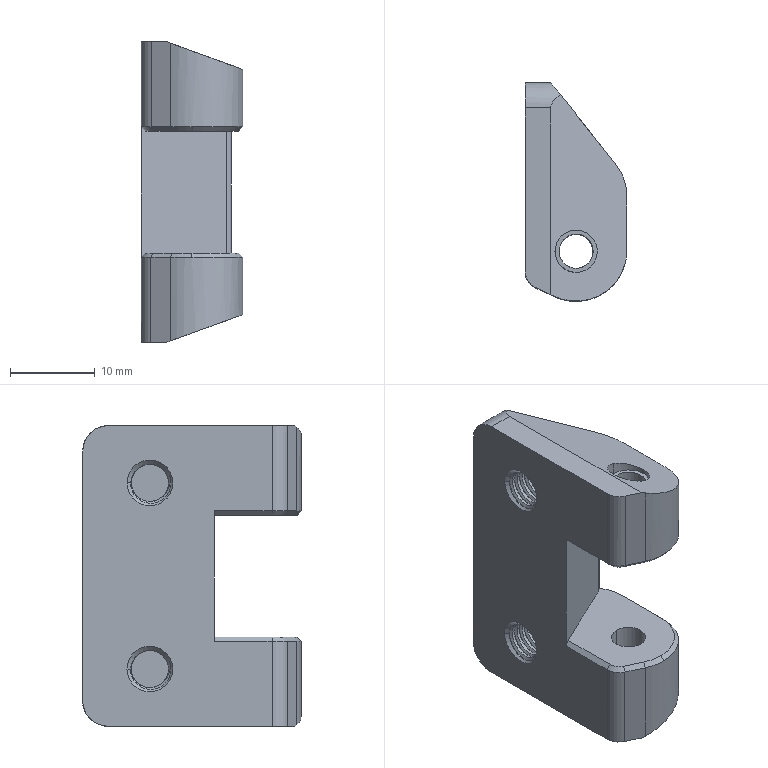Part | SolidWorks | features BaseBody 1 | 1 solid | 142 faces | box 12.027 x 25.816 x 35.476 mm | volume 5447 mm3 | cylinder 90 | plane 30 | cone 18 | spline 4 | commonest cylinder face diameters 5 x44 4.4 x31 4.03 x6 12 x4 4 x2 6 x2